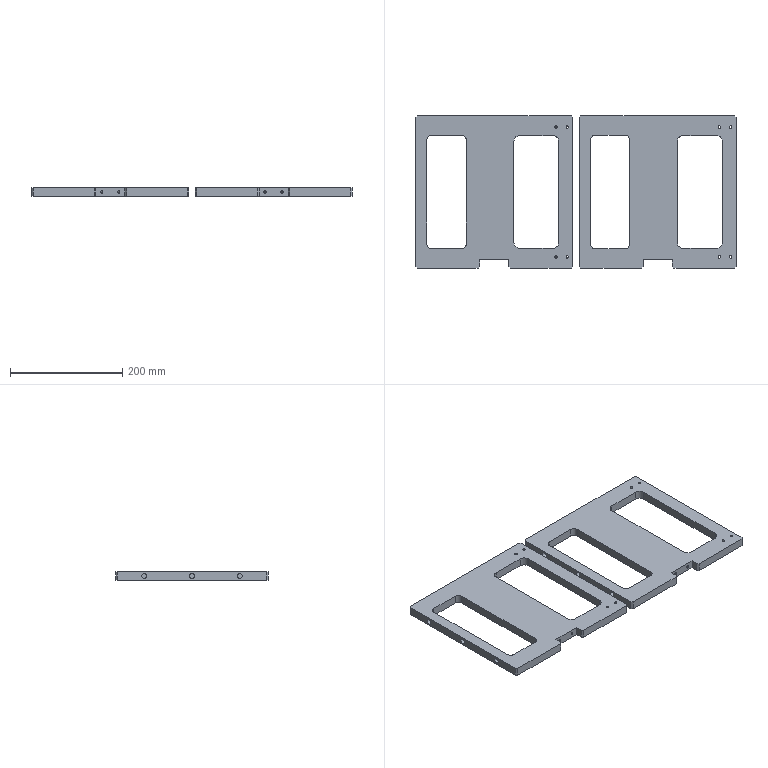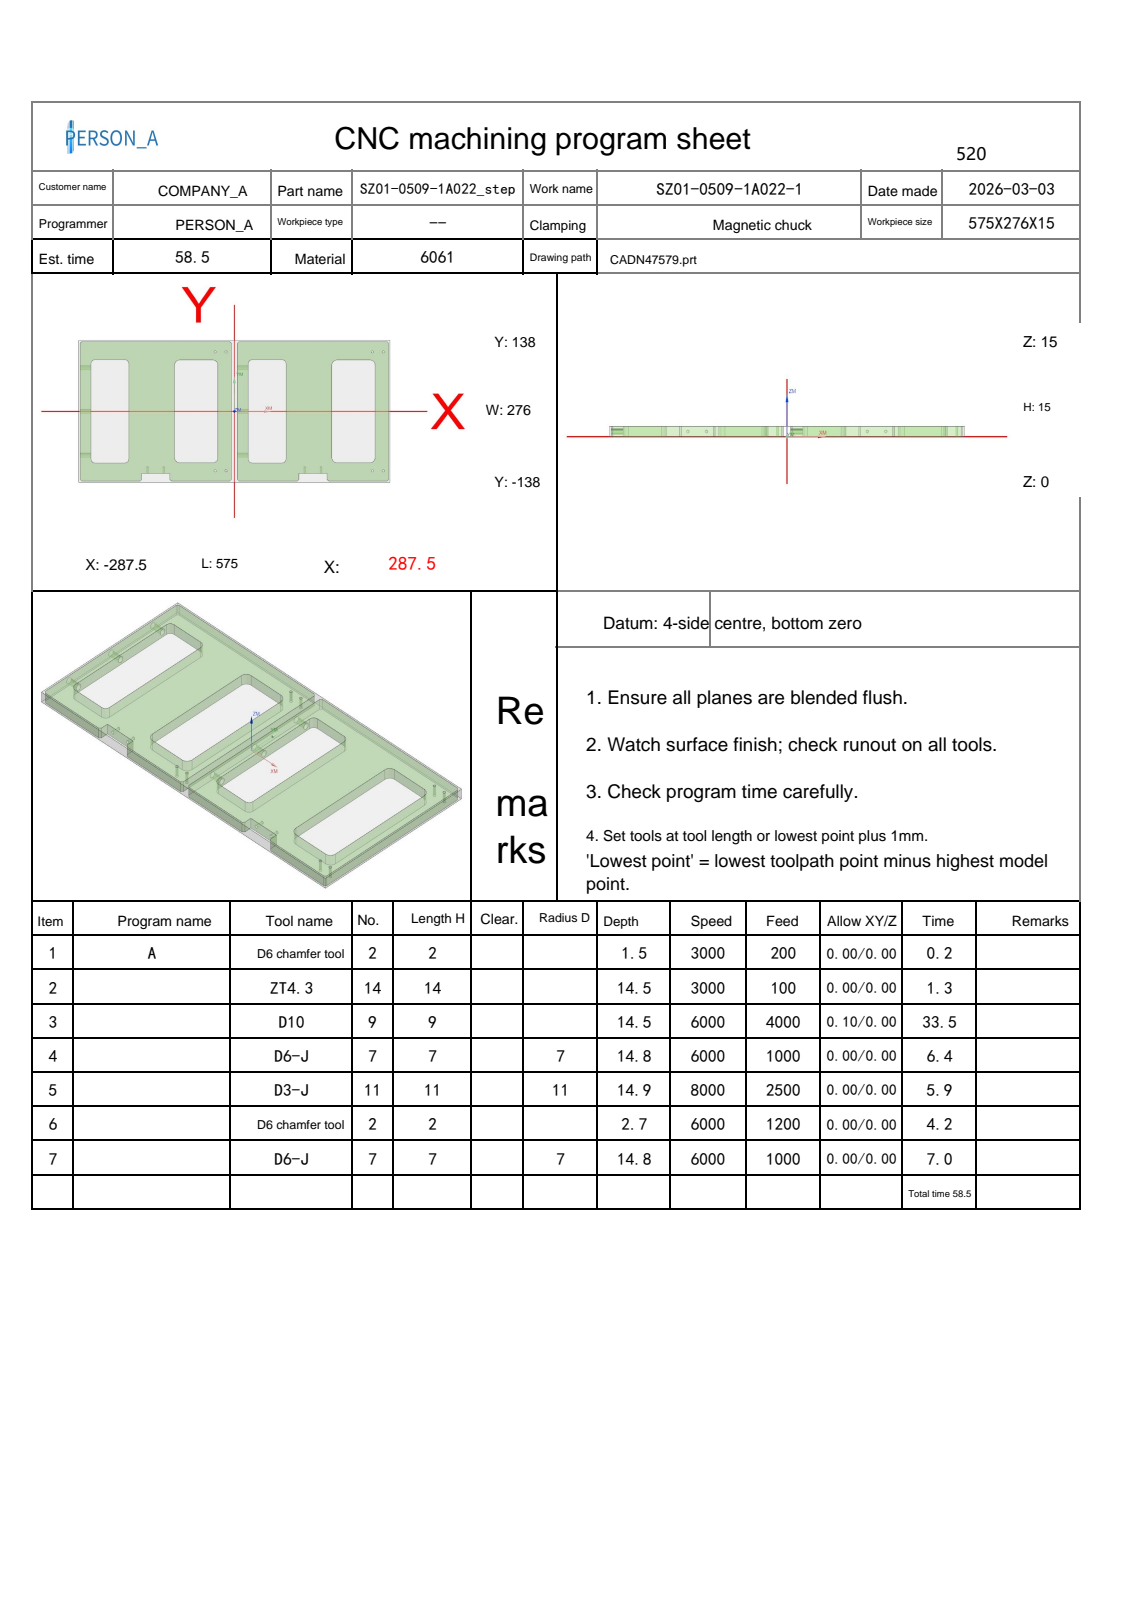NC program | NX | posted by the shop | part box 570 x 271 x 15 mm
Lines 2982 to 3815 of 10286:
N5 T11 M06
(D3-J  D=3. R=0. H=11 ce=0.00 di=0.00)
(D.N=11 MAX_Z=45. MIN_Z=0.15 Time=5.87M)
G00 G90 G54 X-15.613 Y114.911 M03 S8000
G43 H11 Z45.
M08
Z15.5
G01 X-15.578 Y114.9 Z15.498 F300.
X-15.422 Z15.49
X-15.233 Y114.957 Z15.48
X-15.072 Y115.072 Z15.469
X-14.957 Y115.233 Z15.459
X-14.9 Y115.422 Z15.448
Y115.578 Z15.44
X-14.953 Y115.758 Z15.43
X-15.059 Y115.914 Z15.421
X-15.208 Y116.03 Z15.411
X-15.385 Y116.094 Z15.401
X-15.578 Y116.1 Z15.391
X-15.767 Y116.043 Z15.38
X-15.928 Y115.928 Z15.37
X-16.043 Y115.767 Z15.36
X-16.1 Y115.578 Z15.349
Y115.422 Z15.341
X-16.043 Y115.233 Z15.331
X-15.928 Y115.072 Z15.32
X-15.767 Y114.957 Z15.31
X-15.578 Y114.9 Z15.3
X-15.422 Z15.292
X-15.233 Y114.957 Z15.281
X-15.072 Y115.072 Z15.271
X-14.957 Y115.233 Z15.26
X-14.9 Y115.422 Z15.25
Y115.578 Z15.242
X-14.953 Y115.758 Z15.232
X-15.059 Y115.914 Z15.222
X-15.208 Y116.03 Z15.212
X-15.385 Y116.094 Z15.202
X-15.578 Y116.1 Z15.192
X-15.767 Y116.043 Z15.182
X-15.928 Y115.928 Z15.172
X-16.043 Y115.767 Z15.161
X-16.1 Y115.578 Z15.151
Y115.422 Z15.143
X-16.043 Y115.233 Z15.132
X-15.928 Y115.072 Z15.122
X-15.767 Y114.957 Z15.112
X-15.578 Y114.9 Z15.101
X-15.422 Z15.093
X-15.233 Y114.957 Z15.083
X-15.072 Y115.072 Z15.072
X-14.957 Y115.233 Z15.062
X-14.9 Y115.422 Z15.052
Y115.578 Z15.044
X-14.953 Y115.758 Z15.034
X-15.059 Y115.914 Z15.024
X-15.208 Y116.03 Z15.014
X-15.385 Y116.094 Z15.004
X-15.463 Y116.099 Z15.
X-15.465 Y116.065
G41 D11
X-15.5 Y116.1
G03 X-16.1 Y115.5 Z14.914 I0.0 J-.6
X-15.5 Y114.9 Z14.827 I.6 J0.0
X-14.9 Y115.5 Z14.741 I0.0 J.6
X-15.5 Y116.1 Z14.655 I-.6 J0.0
X-16.1 Y115.5 Z14.568 I0.0 J-.6
X-15.5 Y114.9 Z14.482 I.6 J0.0
X-14.9 Y115.5 Z14.396 I0.0 J.6
X-15.5 Y116.1 Z14.309 I-.6 J0.0
X-16.1 Y115.5 Z14.223 I0.0 J-.6
X-15.5 Y114.9 Z14.137 I.6 J0.0
X-14.9 Y115.5 Z14.05 I0.0 J.6
X-15.5 Y116.1 Z13.964 I-.6 J0.0
X-16.1 Y115.5 Z13.878 I0.0 J-.6
X-15.5 Y114.9 Z13.791 I.6 J0.0
X-14.9 Y115.5 Z13.705 I0.0 J.6
X-15.5 Y116.1 Z13.619 I-.6 J0.0
X-16.1 Y115.5 Z13.532 I0.0 J-.6
X-15.5 Y114.9 Z13.446 I.6 J0.0
X-14.9 Y115.5 Z13.36 I0.0 J.6
X-15.5 Y116.1 Z13.273 I-.6 J0.0
X-16.1 Y115.5 Z13.187 I0.0 J-.6
X-15.5 Y114.9 Z13.101 I.6 J0.0
X-14.9 Y115.5 Z13.014 I0.0 J.6
X-15.5 Y116.1 Z12.928 I-.6 J0.0
X-16.1 Y115.5 Z12.842 I0.0 J-.6
X-15.5 Y114.9 Z12.755 I.6 J0.0
X-14.9 Y115.5 Z12.669 I0.0 J.6
X-15.5 Y116.1 Z12.583 I-.6 J0.0
X-16.1 Y115.5 Z12.496 I0.0 J-.6
X-15.5 Y114.9 Z12.41 I.6 J0.0
X-14.9 Y115.5 Z12.324 I0.0 J.6
X-15.5 Y116.1 Z12.237 I-.6 J0.0
X-16.1 Y115.5 Z12.151 I0.0 J-.6
X-15.5 Y114.9 Z12.065 I.6 J0.0
X-14.9 Y115.5 Z11.978 I0.0 J.6
X-15.5 Y116.1 Z11.892 I-.6 J0.0
X-16.1 Y115.5 Z11.806 I0.0 J-.6
X-15.5 Y114.9 Z11.719 I.6 J0.0
X-14.9 Y115.5 Z11.633 I0.0 J.6
X-15.5 Y116.1 Z11.547 I-.6 J0.0
X-16.1 Y115.5 Z11.46 I0.0 J-.6
X-15.5 Y114.9 Z11.374 I.6 J0.0
X-14.9 Y115.5 Z11.288 I0.0 J.6
X-15.5 Y116.1 Z11.201 I-.6 J0.0
X-16.1 Y115.5 Z11.115 I0.0 J-.6
X-15.5 Y114.9 Z11.028 I.6 J0.0
X-14.9 Y115.5 Z10.942 I0.0 J.6
X-15.5 Y116.1 Z10.856 I-.6 J0.0
X-16.1 Y115.5 Z10.769 I0.0 J-.6
X-15.5 Y114.9 Z10.683 I.6 J0.0
X-14.9 Y115.5 Z10.597 I0.0 J.6
X-15.5 Y116.1 Z10.51 I-.6 J0.0
X-16.1 Y115.5 Z10.424 I0.0 J-.6
X-15.5 Y114.9 Z10.338 I.6 J0.0
X-14.9 Y115.5 Z10.251 I0.0 J.6
X-15.5 Y116.1 Z10.165 I-.6 J0.0
X-16.1 Y115.5 Z10.079 I0.0 J-.6
X-15.5 Y114.9 Z9.992 I.6 J0.0
X-14.9 Y115.5 Z9.906 I0.0 J.6
X-15.5 Y116.1 Z9.82 I-.6 J0.0
X-16.1 Y115.5 Z9.733 I0.0 J-.6
X-15.5 Y114.9 Z9.647 I.6 J0.0
X-14.9 Y115.5 Z9.561 I0.0 J.6
X-15.5 Y116.1 Z9.474 I-.6 J0.0
X-16.1 Y115.5 Z9.388 I0.0 J-.6
X-15.5 Y114.9 Z9.302 I.6 J0.0
X-14.9 Y115.5 Z9.215 I0.0 J.6
X-15.5 Y116.1 Z9.129 I-.6 J0.0
X-16.1 Y115.5 Z9.043 I0.0 J-.6
X-15.5 Y114.9 Z8.956 I.6 J0.0
X-14.9 Y115.5 Z8.87 I0.0 J.6
X-15.5 Y116.1 Z8.784 I-.6 J0.0
X-16.1 Y115.5 Z8.697 I0.0 J-.6
X-15.5 Y114.9 Z8.611 I.6 J0.0
X-14.9 Y115.5 Z8.525 I0.0 J.6
X-15.5 Y116.1 Z8.438 I-.6 J0.0
X-16.1 Y115.5 Z8.352 I0.0 J-.6
X-15.5 Y114.9 Z8.266 I.6 J0.0
X-14.9 Y115.5 Z8.179 I0.0 J.6
X-15.5 Y116.1 Z8.093 I-.6 J0.0
X-16.1 Y115.5 Z8.007 I0.0 J-.6
X-15.5 Y114.9 Z7.92 I.6 J0.0
X-14.9 Y115.5 Z7.834 I0.0 J.6
X-15.5 Y116.1 Z7.748 I-.6 J0.0
X-16.1 Y115.5 Z7.661 I0.0 J-.6
X-15.5 Y114.9 Z7.575 I.6 J0.0
X-14.9 Y115.5 Z7.489 I0.0 J.6
X-15.5 Y116.1 Z7.402 I-.6 J0.0
X-16.1 Y115.5 Z7.316 I0.0 J-.6
X-15.5 Y114.9 Z7.23 I.6 J0.0
X-14.9 Y115.5 Z7.143 I0.0 J.6
X-15.5 Y116.1 Z7.057 I-.6 J0.0
X-16.1 Y115.5 Z6.971 I0.0 J-.6
X-15.5 Y114.9 Z6.884 I.6 J0.0
X-14.9 Y115.5 Z6.798 I0.0 J.6
X-15.5 Y116.1 Z6.712 I-.6 J0.0
X-16.1 Y115.5 Z6.625 I0.0 J-.6
X-15.5 Y114.9 Z6.539 I.6 J0.0
X-14.9 Y115.5 Z6.453 I0.0 J.6
X-15.5 Y116.1 Z6.366 I-.6 J0.0
X-16.1 Y115.5 Z6.28 I0.0 J-.6
X-15.5 Y114.9 Z6.194 I.6 J0.0
X-14.9 Y115.5 Z6.107 I0.0 J.6
X-15.5 Y116.1 Z6.021 I-.6 J0.0
X-16.1 Y115.5 Z5.935 I0.0 J-.6
X-15.5 Y114.9 Z5.848 I.6 J0.0
X-14.9 Y115.5 Z5.762 I0.0 J.6
X-15.5 Y116.1 Z5.676 I-.6 J0.0
X-16.1 Y115.5 Z5.589 I0.0 J-.6
X-15.5 Y114.9 Z5.503 I.6 J0.0
X-14.9 Y115.5 Z5.417 I0.0 J.6
X-15.5 Y116.1 Z5.33 I-.6 J0.0
X-16.1 Y115.5 Z5.244 I0.0 J-.6
X-15.5 Y114.9 Z5.158 I.6 J0.0
X-14.9 Y115.5 Z5.071 I0.0 J.6
X-15.5 Y116.1 Z4.985 I-.6 J0.0
X-16.1 Y115.5 Z4.899 I0.0 J-.6
X-15.5 Y114.9 Z4.812 I.6 J0.0
X-14.9 Y115.5 Z4.726 I0.0 J.6
X-15.5 Y116.1 Z4.64 I-.6 J0.0
X-16.1 Y115.5 Z4.553 I0.0 J-.6
X-15.5 Y114.9 Z4.467 I.6 J0.0
X-14.9 Y115.5 Z4.381 I0.0 J.6
X-15.5 Y116.1 Z4.294 I-.6 J0.0
X-16.1 Y115.5 Z4.208 I0.0 J-.6
X-15.5 Y114.9 Z4.122 I.6 J0.0
X-14.9 Y115.5 Z4.035 I0.0 J.6
X-15.5 Y116.1 Z3.949 I-.6 J0.0
X-16.1 Y115.5 Z3.863 I0.0 J-.6
X-15.5 Y114.9 Z3.776 I.6 J0.0
X-14.9 Y115.5 Z3.69 I0.0 J.6
X-15.5 Y116.1 Z3.603 I-.6 J0.0
X-16.1 Y115.5 Z3.517 I0.0 J-.6
X-15.5 Y114.9 Z3.431 I.6 J0.0
X-14.9 Y115.5 Z3.344 I0.0 J.6
X-15.5 Y116.1 Z3.258 I-.6 J0.0
X-16.1 Y115.5 Z3.172 I0.0 J-.6
X-15.5 Y114.9 Z3.085 I.6 J0.0
X-14.9 Y115.5 Z2.999 I0.0 J.6
X-15.5 Y116.1 Z2.913 I-.6 J0.0
X-16.1 Y115.5 Z2.826 I0.0 J-.6
X-15.5 Y114.9 Z2.74 I.6 J0.0
X-14.9 Y115.5 Z2.654 I0.0 J.6
X-15.5 Y116.1 Z2.567 I-.6 J0.0
X-16.1 Y115.5 Z2.481 I0.0 J-.6
X-15.5 Y114.9 Z2.395 I.6 J0.0
X-14.9 Y115.5 Z2.308 I0.0 J.6
X-15.5 Y116.1 Z2.222 I-.6 J0.0
X-16.1 Y115.5 Z2.136 I0.0 J-.6
X-15.5 Y114.9 Z2.049 I.6 J0.0
X-14.9 Y115.5 Z1.963 I0.0 J.6
X-15.5 Y116.1 Z1.877 I-.6 J0.0
X-16.1 Y115.5 Z1.79 I0.0 J-.6
X-15.5 Y114.9 Z1.704 I.6 J0.0
X-14.9 Y115.5 Z1.618 I0.0 J.6
X-15.5 Y116.1 Z1.531 I-.6 J0.0
X-16.1 Y115.5 Z1.445 I0.0 J-.6
X-15.5 Y114.9 Z1.359 I.6 J0.0
X-14.9 Y115.5 Z1.272 I0.0 J.6
X-15.5 Y116.1 Z1.186 I-.6 J0.0
X-16.1 Y115.5 Z1.1 I0.0 J-.6
X-15.5 Y114.9 Z1.013 I.6 J0.0
X-14.9 Y115.5 Z.927 I0.0 J.6
X-15.5 Y116.1 Z.841 I-.6 J0.0
X-16.1 Y115.5 Z.754 I0.0 J-.6
X-15.5 Y114.9 Z.668 I.6 J0.0
X-14.9 Y115.5 Z.582 I0.0 J.6
X-15.5 Y116.1 Z.495 I-.6 J0.0
X-16.1 Y115.5 Z.409 I0.0 J-.6
X-15.5 Y114.9 Z.323 I.6 J0.0
X-14.9 Y115.5 Z.236 I0.0 J.6
X-15.5 Y116.1 Z.15 I-.6 J0.0
X-16.1 Y115.5 I0.0 J-.6
X-15.5 Y114.9 I.6 J0.0
X-14.9 Y115.5 I0.0 J.6
X-15.5 Y116.1 I-.6 J0.0
X-15.871 Y115.972 I0.0 J-.6
G01 X-15.891 Y115.953
X-15.895 Y115.924
X-15.879 Y115.901
G40 X-15.848 Y115.862
Z1.15
G00 Z45.
X-35.613 Y114.911
Z15.5
G01 X-35.578 Y114.9 Z15.498
X-35.422 Z15.49
X-35.233 Y114.957 Z15.48
X-35.072 Y115.072 Z15.469
X-34.957 Y115.233 Z15.459
X-34.9 Y115.422 Z15.448
Y115.578 Z15.44
X-34.953 Y115.758 Z15.43
X-35.059 Y115.914 Z15.421
X-35.208 Y116.03 Z15.411
X-35.385 Y116.094 Z15.401
X-35.578 Y116.1 Z15.391
X-35.767 Y116.043 Z15.38
X-35.928 Y115.928 Z15.37
X-36.043 Y115.767 Z15.36
X-36.1 Y115.578 Z15.349
Y115.422 Z15.341
X-36.043 Y115.233 Z15.331
X-35.928 Y115.072 Z15.32
X-35.767 Y114.957 Z15.31
X-35.578 Y114.9 Z15.3
X-35.422 Z15.292
X-35.233 Y114.957 Z15.281
X-35.072 Y115.072 Z15.271
X-34.957 Y115.233 Z15.26
X-34.9 Y115.422 Z15.25
Y115.578 Z15.242
X-34.953 Y115.758 Z15.232
X-35.059 Y115.914 Z15.222
X-35.208 Y116.03 Z15.212
X-35.385 Y116.094 Z15.202
X-35.578 Y116.1 Z15.192
X-35.767 Y116.043 Z15.182
X-35.928 Y115.928 Z15.172
X-36.043 Y115.767 Z15.161
X-36.1 Y115.578 Z15.151
Y115.422 Z15.143
X-36.043 Y115.233 Z15.132
X-35.928 Y115.072 Z15.122
X-35.767 Y114.957 Z15.112
X-35.578 Y114.9 Z15.101
X-35.422 Z15.093
X-35.233 Y114.957 Z15.083
X-35.072 Y115.072 Z15.072
X-34.957 Y115.233 Z15.062
X-34.9 Y115.422 Z15.052
Y115.578 Z15.044
X-34.953 Y115.758 Z15.034
X-35.059 Y115.914 Z15.024
X-35.208 Y116.03 Z15.014
X-35.385 Y116.094 Z15.004
X-35.463 Y116.099 Z15.
X-35.465 Y116.065
G41 D11
X-35.5 Y116.1
G03 X-36.1 Y115.5 Z14.914 I0.0 J-.6
X-35.5 Y114.9 Z14.827 I.6 J0.0
X-34.9 Y115.5 Z14.741 I0.0 J.6
X-35.5 Y116.1 Z14.655 I-.6 J0.0
X-36.1 Y115.5 Z14.568 I0.0 J-.6
X-35.5 Y114.9 Z14.482 I.6 J0.0
X-34.9 Y115.5 Z14.396 I0.0 J.6
X-35.5 Y116.1 Z14.309 I-.6 J0.0
X-36.1 Y115.5 Z14.223 I0.0 J-.6
X-35.5 Y114.9 Z14.137 I.6 J0.0
X-34.9 Y115.5 Z14.05 I0.0 J.6
X-35.5 Y116.1 Z13.964 I-.6 J0.0
X-36.1 Y115.5 Z13.878 I0.0 J-.6
X-35.5 Y114.9 Z13.791 I.6 J0.0
X-34.9 Y115.5 Z13.705 I0.0 J.6
X-35.5 Y116.1 Z13.619 I-.6 J0.0
X-36.1 Y115.5 Z13.532 I0.0 J-.6
X-35.5 Y114.9 Z13.446 I.6 J0.0
X-34.9 Y115.5 Z13.36 I0.0 J.6
X-35.5 Y116.1 Z13.273 I-.6 J0.0
X-36.1 Y115.5 Z13.187 I0.0 J-.6
X-35.5 Y114.9 Z13.101 I.6 J0.0
X-34.9 Y115.5 Z13.014 I0.0 J.6
X-35.5 Y116.1 Z12.928 I-.6 J0.0
X-36.1 Y115.5 Z12.842 I0.0 J-.6
X-35.5 Y114.9 Z12.755 I.6 J0.0
X-34.9 Y115.5 Z12.669 I0.0 J.6
X-35.5 Y116.1 Z12.583 I-.6 J0.0
X-36.1 Y115.5 Z12.496 I0.0 J-.6
X-35.5 Y114.9 Z12.41 I.6 J0.0
X-34.9 Y115.5 Z12.324 I0.0 J.6
X-35.5 Y116.1 Z12.237 I-.6 J0.0
X-36.1 Y115.5 Z12.151 I0.0 J-.6
X-35.5 Y114.9 Z12.065 I.6 J0.0
X-34.9 Y115.5 Z11.978 I0.0 J.6
X-35.5 Y116.1 Z11.892 I-.6 J0.0
X-36.1 Y115.5 Z11.806 I0.0 J-.6
X-35.5 Y114.9 Z11.719 I.6 J0.0
X-34.9 Y115.5 Z11.633 I0.0 J.6
X-35.5 Y116.1 Z11.547 I-.6 J0.0
X-36.1 Y115.5 Z11.46 I0.0 J-.6
X-35.5 Y114.9 Z11.374 I.6 J0.0
X-34.9 Y115.5 Z11.288 I0.0 J.6
X-35.5 Y116.1 Z11.201 I-.6 J0.0
X-36.1 Y115.5 Z11.115 I0.0 J-.6
X-35.5 Y114.9 Z11.028 I.6 J0.0
X-34.9 Y115.5 Z10.942 I0.0 J.6
X-35.5 Y116.1 Z10.856 I-.6 J0.0
X-36.1 Y115.5 Z10.769 I0.0 J-.6
X-35.5 Y114.9 Z10.683 I.6 J0.0
X-34.9 Y115.5 Z10.597 I0.0 J.6
X-35.5 Y116.1 Z10.51 I-.6 J0.0
X-36.1 Y115.5 Z10.424 I0.0 J-.6
X-35.5 Y114.9 Z10.338 I.6 J0.0
X-34.9 Y115.5 Z10.251 I0.0 J.6
X-35.5 Y116.1 Z10.165 I-.6 J0.0
X-36.1 Y115.5 Z10.079 I0.0 J-.6
X-35.5 Y114.9 Z9.992 I.6 J0.0
X-34.9 Y115.5 Z9.906 I0.0 J.6
X-35.5 Y116.1 Z9.82 I-.6 J0.0
X-36.1 Y115.5 Z9.733 I0.0 J-.6
X-35.5 Y114.9 Z9.647 I.6 J0.0
X-34.9 Y115.5 Z9.561 I0.0 J.6
X-35.5 Y116.1 Z9.474 I-.6 J0.0
X-36.1 Y115.5 Z9.388 I0.0 J-.6
X-35.5 Y114.9 Z9.302 I.6 J0.0
X-34.9 Y115.5 Z9.215 I0.0 J.6
X-35.5 Y116.1 Z9.129 I-.6 J0.0
X-36.1 Y115.5 Z9.043 I0.0 J-.6
X-35.5 Y114.9 Z8.956 I.6 J0.0
X-34.9 Y115.5 Z8.87 I0.0 J.6
X-35.5 Y116.1 Z8.784 I-.6 J0.0
X-36.1 Y115.5 Z8.697 I0.0 J-.6
X-35.5 Y114.9 Z8.611 I.6 J0.0
X-34.9 Y115.5 Z8.525 I0.0 J.6
X-35.5 Y116.1 Z8.438 I-.6 J0.0
X-36.1 Y115.5 Z8.352 I0.0 J-.6
X-35.5 Y114.9 Z8.266 I.6 J0.0
X-34.9 Y115.5 Z8.179 I0.0 J.6
X-35.5 Y116.1 Z8.093 I-.6 J0.0
X-36.1 Y115.5 Z8.007 I0.0 J-.6
X-35.5 Y114.9 Z7.92 I.6 J0.0
X-34.9 Y115.5 Z7.834 I0.0 J.6
X-35.5 Y116.1 Z7.748 I-.6 J0.0
X-36.1 Y115.5 Z7.661 I0.0 J-.6
X-35.5 Y114.9 Z7.575 I.6 J0.0
X-34.9 Y115.5 Z7.489 I0.0 J.6
X-35.5 Y116.1 Z7.402 I-.6 J0.0
X-36.1 Y115.5 Z7.316 I0.0 J-.6
X-35.5 Y114.9 Z7.23 I.6 J0.0
X-34.9 Y115.5 Z7.143 I0.0 J.6
X-35.5 Y116.1 Z7.057 I-.6 J0.0
X-36.1 Y115.5 Z6.971 I0.0 J-.6
X-35.5 Y114.9 Z6.884 I.6 J0.0
X-34.9 Y115.5 Z6.798 I0.0 J.6
X-35.5 Y116.1 Z6.712 I-.6 J0.0
X-36.1 Y115.5 Z6.625 I0.0 J-.6
X-35.5 Y114.9 Z6.539 I.6 J0.0
X-34.9 Y115.5 Z6.453 I0.0 J.6
X-35.5 Y116.1 Z6.366 I-.6 J0.0
X-36.1 Y115.5 Z6.28 I0.0 J-.6
X-35.5 Y114.9 Z6.194 I.6 J0.0
X-34.9 Y115.5 Z6.107 I0.0 J.6
X-35.5 Y116.1 Z6.021 I-.6 J0.0
X-36.1 Y115.5 Z5.935 I0.0 J-.6
X-35.5 Y114.9 Z5.848 I.6 J0.0
X-34.9 Y115.5 Z5.762 I0.0 J.6
X-35.5 Y116.1 Z5.676 I-.6 J0.0
X-36.1 Y115.5 Z5.589 I0.0 J-.6
X-35.5 Y114.9 Z5.503 I.6 J0.0
X-34.9 Y115.5 Z5.417 I0.0 J.6
X-35.5 Y116.1 Z5.33 I-.6 J0.0
X-36.1 Y115.5 Z5.244 I0.0 J-.6
X-35.5 Y114.9 Z5.158 I.6 J0.0
X-34.9 Y115.5 Z5.071 I0.0 J.6
X-35.5 Y116.1 Z4.985 I-.6 J0.0
X-36.1 Y115.5 Z4.899 I0.0 J-.6
X-35.5 Y114.9 Z4.812 I.6 J0.0
X-34.9 Y115.5 Z4.726 I0.0 J.6
X-35.5 Y116.1 Z4.64 I-.6 J0.0
X-36.1 Y115.5 Z4.553 I0.0 J-.6
X-35.5 Y114.9 Z4.467 I.6 J0.0
X-34.9 Y115.5 Z4.381 I0.0 J.6
X-35.5 Y116.1 Z4.294 I-.6 J0.0
X-36.1 Y115.5 Z4.208 I0.0 J-.6
X-35.5 Y114.9 Z4.122 I.6 J0.0
X-34.9 Y115.5 Z4.035 I0.0 J.6
X-35.5 Y116.1 Z3.949 I-.6 J0.0
X-36.1 Y115.5 Z3.863 I0.0 J-.6
X-35.5 Y114.9 Z3.776 I.6 J0.0
X-34.9 Y115.5 Z3.69 I0.0 J.6
X-35.5 Y116.1 Z3.603 I-.6 J0.0
X-36.1 Y115.5 Z3.517 I0.0 J-.6
X-35.5 Y114.9 Z3.431 I.6 J0.0
X-34.9 Y115.5 Z3.344 I0.0 J.6
X-35.5 Y116.1 Z3.258 I-.6 J0.0
X-36.1 Y115.5 Z3.172 I0.0 J-.6
X-35.5 Y114.9 Z3.085 I.6 J0.0
X-34.9 Y115.5 Z2.999 I0.0 J.6
X-35.5 Y116.1 Z2.913 I-.6 J0.0
X-36.1 Y115.5 Z2.826 I0.0 J-.6
X-35.5 Y114.9 Z2.74 I.6 J0.0
X-34.9 Y115.5 Z2.654 I0.0 J.6
X-35.5 Y116.1 Z2.567 I-.6 J0.0
X-36.1 Y115.5 Z2.481 I0.0 J-.6
X-35.5 Y114.9 Z2.395 I.6 J0.0
X-34.9 Y115.5 Z2.308 I0.0 J.6
X-35.5 Y116.1 Z2.222 I-.6 J0.0
X-36.1 Y115.5 Z2.136 I0.0 J-.6
X-35.5 Y114.9 Z2.049 I.6 J0.0
X-34.9 Y115.5 Z1.963 I0.0 J.6
X-35.5 Y116.1 Z1.877 I-.6 J0.0
X-36.1 Y115.5 Z1.79 I0.0 J-.6
X-35.5 Y114.9 Z1.704 I.6 J0.0
X-34.9 Y115.5 Z1.618 I0.0 J.6
X-35.5 Y116.1 Z1.531 I-.6 J0.0
X-36.1 Y115.5 Z1.445 I0.0 J-.6
X-35.5 Y114.9 Z1.359 I.6 J0.0
X-34.9 Y115.5 Z1.272 I0.0 J.6
X-35.5 Y116.1 Z1.186 I-.6 J0.0
X-36.1 Y115.5 Z1.1 I0.0 J-.6
X-35.5 Y114.9 Z1.013 I.6 J0.0
X-34.9 Y115.5 Z.927 I0.0 J.6
X-35.5 Y116.1 Z.841 I-.6 J0.0
X-36.1 Y115.5 Z.754 I0.0 J-.6
X-35.5 Y114.9 Z.668 I.6 J0.0
X-34.9 Y115.5 Z.582 I0.0 J.6
X-35.5 Y116.1 Z.495 I-.6 J0.0
X-36.1 Y115.5 Z.409 I0.0 J-.6
X-35.5 Y114.9 Z.323 I.6 J0.0
X-34.9 Y115.5 Z.236 I0.0 J.6
X-35.5 Y116.1 Z.15 I-.6 J0.0
X-36.1 Y115.5 I0.0 J-.6
X-35.5 Y114.9 I.6 J0.0
X-34.9 Y115.5 I0.0 J.6
X-35.5 Y116.1 I-.6 J0.0
X-35.871 Y115.972 I0.0 J-.6
G01 X-35.891 Y115.953
X-35.895 Y115.924
X-35.879 Y115.901
G40 X-35.848 Y115.862
Z1.15
G00 Z45.
X-35.39 Y-114.91
Z15.5
G01 X-35.422 Y-114.9 Z15.498
X-35.578 Z15.49
X-35.767 Y-114.957 Z15.48
X-35.928 Y-115.072 Z15.469
X-36.043 Y-115.233 Z15.459
X-36.1 Y-115.422 Z15.449
Y-115.578 Z15.441
X-36.069 Y-115.707 Z15.434
X-36.01 Y-115.826 Z15.427
X-35.91 Y-115.945 Z15.418
X-35.773 Y-116.04 Z15.41
X-35.615 Y-116.094 Z15.401
X-35.422 Y-116.1 Z15.391
X-35.233 Y-116.043 Z15.38
X-35.072 Y-115.928 Z15.37
X-34.957 Y-115.767 Z15.36
X-34.9 Y-115.578 Z15.349
Y-115.422 Z15.341
X-34.957 Y-115.233 Z15.331
X-35.072 Y-115.072 Z15.321
X-35.233 Y-114.957 Z15.31
X-35.422 Y-114.9 Z15.3
X-35.578 Z15.292
X-35.767 Y-114.957 Z15.281
X-35.928 Y-115.072 Z15.271
X-36.043 Y-115.233 Z15.261
X-36.1 Y-115.422 Z15.25
Y-115.578 Z15.242
X-36.069 Y-115.707 Z15.235
X-36.01 Y-115.826 Z15.228
X-35.91 Y-115.945 Z15.22
X-35.773 Y-116.04 Z15.211
X-35.615 Y-116.094 Z15.203
X-35.422 Y-116.1 Z15.192
X-35.233 Y-116.043 Z15.182
X-35.072 Y-115.928 Z15.172
X-34.957 Y-115.767 Z15.161
X-34.9 Y-115.578 Z15.151
Y-115.422 Z15.143
X-34.957 Y-115.233 Z15.132
X-35.072 Y-115.072 Z15.122
X-35.233 Y-114.957 Z15.112
X-35.422 Y-114.9 Z15.101
X-35.578 Z15.093
X-35.767 Y-114.957 Z15.083
X-35.928 Y-115.072 Z15.072
X-36.043 Y-115.233 Z15.062
X-36.1 Y-115.422 Z15.052
Y-115.578 Z15.044
X-36.069 Y-115.707 Z15.037
X-36.01 Y-115.826 Z15.03
X-35.91 Y-115.945 Z15.022
X-35.773 Y-116.04 Z15.013
X-35.615 Y-116.094 Z15.004
X-35.537 Y-116.099 Z15.
X-35.535 Y-116.065
G41 D11
X-35.5 Y-116.1
G03 X-34.9 Y-115.5 Z14.914 I0.0 J.6
X-35.5 Y-114.9 Z14.827 I-.6 J0.0
X-36.1 Y-115.5 Z14.741 I0.0 J-.6
X-35.96 Y-115.885 Z14.703 I.6 J0.0
X-35.5 Y-116.1 Z14.655 I.46 J.385
X-34.9 Y-115.5 Z14.568 I0.0 J.6
X-35.5 Y-114.9 Z14.482 I-.6 J0.0
X-36.1 Y-115.5 Z14.396 I0.0 J-.6
X-35.96 Y-115.885 Z14.357 I.6 J0.0
X-35.5 Y-116.1 Z14.309 I.46 J.385
X-34.9 Y-115.5 Z14.223 I0.0 J.6
X-35.5 Y-114.9 Z14.137 I-.6 J0.0
X-36.1 Y-115.5 Z14.05 I0.0 J-.6
X-35.96 Y-115.885 Z14.012 I.6 J0.0
X-35.5 Y-116.1 Z13.964 I.46 J.385
X-34.9 Y-115.5 Z13.878 I0.0 J.6
X-35.5 Y-114.9 Z13.791 I-.6 J0.0
X-36.1 Y-115.5 Z13.705 I0.0 J-.6
X-35.96 Y-115.885 Z13.667 I.6 J0.0
X-35.5 Y-116.1 Z13.619 I.46 J.385
X-34.9 Y-115.5 Z13.532 I0.0 J.6
X-35.5 Y-114.9 Z13.446 I-.6 J0.0
X-36.1 Y-115.5 Z13.36 I0.0 J-.6
X-35.96 Y-115.885 Z13.321 I.6 J0.0
X-35.5 Y-116.1 Z13.273 I.46 J.385
X-34.9 Y-115.5 Z13.187 I0.0 J.6
X-35.5 Y-114.9 Z13.101 I-.6 J0.0
X-36.1 Y-115.5 Z13.014 I0.0 J-.6
X-35.96 Y-115.885 Z12.976 I.6 J0.0
X-35.5 Y-116.1 Z12.928 I.46 J.385
X-34.9 Y-115.5 Z12.842 I0.0 J.6
X-35.5 Y-114.9 Z12.755 I-.6 J0.0
X-36.1 Y-115.5 Z12.669 I0.0 J-.6
X-35.96 Y-115.885 Z12.631 I.6 J0.0
X-35.5 Y-116.1 Z12.583 I.46 J.385
X-34.9 Y-115.5 Z12.496 I0.0 J.6
X-35.5 Y-114.9 Z12.41 I-.6 J0.0
X-36.1 Y-115.5 Z12.324 I0.0 J-.6
X-35.96 Y-115.885 Z12.285 I.6 J0.0
X-35.5 Y-116.1 Z12.237 I.46 J.385
X-34.9 Y-115.5 Z12.151 I0.0 J.6
X-35.5 Y-114.9 Z12.065 I-.6 J0.0
X-36.1 Y-115.5 Z11.978 I0.0 J-.6
X-35.96 Y-115.885 Z11.94 I.6 J0.0
X-35.5 Y-116.1 Z11.892 I.46 J.385
X-34.9 Y-115.5 Z11.806 I0.0 J.6
X-35.5 Y-114.9 Z11.719 I-.6 J0.0
X-36.1 Y-115.5 Z11.633 I0.0 J-.6
X-35.96 Y-115.885 Z11.595 I.6 J0.0
X-35.5 Y-116.1 Z11.547 I.46 J.385
X-34.9 Y-115.5 Z11.46 I0.0 J.6
X-35.5 Y-114.9 Z11.374 I-.6 J0.0
X-36.1 Y-115.5 Z11.288 I0.0 J-.6
X-35.96 Y-115.885 Z11.249 I.6 J0.0
X-35.5 Y-116.1 Z11.201 I.46 J.385
X-34.9 Y-115.5 Z11.115 I0.0 J.6
X-35.5 Y-114.9 Z11.028 I-.6 J0.0
X-36.1 Y-115.5 Z10.942 I0.0 J-.6
X-35.96 Y-115.885 Z10.904 I.6 J0.0
X-35.5 Y-116.1 Z10.856 I.46 J.385
X-34.9 Y-115.5 Z10.769 I0.0 J.6
X-35.5 Y-114.9 Z10.683 I-.6 J0.0
X-36.1 Y-115.5 Z10.597 I0.0 J-.6
X-35.96 Y-115.885 Z10.559 I.6 J0.0
X-35.5 Y-116.1 Z10.51 I.46 J.385
X-34.9 Y-115.5 Z10.424 I0.0 J.6
X-35.5 Y-114.9 Z10.338 I-.6 J0.0
X-36.1 Y-115.5 Z10.251 I0.0 J-.6
X-35.96 Y-115.885 Z10.213 I.6 J0.0
X-35.5 Y-116.1 Z10.165 I.46 J.385
X-34.9 Y-115.5 Z10.079 I0.0 J.6
X-35.5 Y-114.9 Z9.992 I-.6 J0.0
X-36.1 Y-115.5 Z9.906 I0.0 J-.6
X-35.96 Y-115.885 Z9.868 I.6 J0.0
X-35.5 Y-116.1 Z9.82 I.46 J.385
X-34.9 Y-115.5 Z9.733 I0.0 J.6
X-35.5 Y-114.9 Z9.647 I-.6 J0.0
X-36.1 Y-115.5 Z9.561 I0.0 J-.6
X-35.96 Y-115.885 Z9.522 I.6 J0.0
X-35.5 Y-116.1 Z9.474 I.46 J.385
X-34.9 Y-115.5 Z9.388 I0.0 J.6
X-35.5 Y-114.9 Z9.302 I-.6 J0.0
X-36.1 Y-115.5 Z9.215 I0.0 J-.6
X-35.96 Y-115.885 Z9.177 I.6 J0.0
X-35.5 Y-116.1 Z9.129 I.46 J.385
X-34.9 Y-115.5 Z9.043 I0.0 J.6
X-35.5 Y-114.9 Z8.956 I-.6 J0.0
X-36.1 Y-115.5 Z8.87 I0.0 J-.6
X-35.96 Y-115.885 Z8.832 I.6 J0.0
X-35.5 Y-116.1 Z8.784 I.46 J.385
X-34.9 Y-115.5 Z8.697 I0.0 J.6
X-35.5 Y-114.9 Z8.611 I-.6 J0.0
X-36.1 Y-115.5 Z8.525 I0.0 J-.6
X-35.96 Y-115.885 Z8.486 I.6 J0.0
X-35.5 Y-116.1 Z8.438 I.46 J.385
X-34.9 Y-115.5 Z8.352 I0.0 J.6
X-35.5 Y-114.9 Z8.266 I-.6 J0.0
X-36.1 Y-115.5 Z8.179 I0.0 J-.6
X-35.96 Y-115.885 Z8.141 I.6 J0.0
X-35.5 Y-116.1 Z8.093 I.46 J.385
X-34.9 Y-115.5 Z8.007 I0.0 J.6
X-35.5 Y-114.9 Z7.92 I-.6 J0.0
X-36.1 Y-115.5 Z7.834 I0.0 J-.6
X-35.96 Y-115.885 Z7.796 I.6 J0.0
X-35.5 Y-116.1 Z7.748 I.46 J.385
X-34.9 Y-115.5 Z7.661 I0.0 J.6
X-35.5 Y-114.9 Z7.575 I-.6 J0.0
X-36.1 Y-115.5 Z7.489 I0.0 J-.6
X-35.96 Y-115.885 Z7.45 I.6 J0.0
X-35.5 Y-116.1 Z7.402 I.46 J.385
X-34.9 Y-115.5 Z7.316 I0.0 J.6
X-35.5 Y-114.9 Z7.23 I-.6 J0.0
X-36.1 Y-115.5 Z7.143 I0.0 J-.6
X-35.96 Y-115.885 Z7.105 I.6 J0.0
X-35.5 Y-116.1 Z7.057 I.46 J.385
X-34.9 Y-115.5 Z6.971 I0.0 J.6
X-35.5 Y-114.9 Z6.884 I-.6 J0.0
X-36.1 Y-115.5 Z6.798 I0.0 J-.6
X-35.96 Y-115.885 Z6.76 I.6 J0.0
X-35.5 Y-116.1 Z6.712 I.46 J.385
X-34.9 Y-115.5 Z6.625 I0.0 J.6
X-35.5 Y-114.9 Z6.539 I-.6 J0.0
X-36.1 Y-115.5 Z6.453 I0.0 J-.6
X-35.96 Y-115.885 Z6.414 I.6 J0.0
X-35.5 Y-116.1 Z6.366 I.46 J.385
X-34.9 Y-115.5 Z6.28 I0.0 J.6
X-35.5 Y-114.9 Z6.194 I-.6 J0.0
X-36.1 Y-115.5 Z6.107 I0.0 J-.6
X-35.96 Y-115.885 Z6.069 I.6 J0.0
X-35.5 Y-116.1 Z6.021 I.46 J.385
X-34.9 Y-115.5 Z5.935 I0.0 J.6
X-35.5 Y-114.9 Z5.848 I-.6 J0.0
X-36.1 Y-115.5 Z5.762 I0.0 J-.6
X-35.96 Y-115.885 Z5.724 I.6 J0.0
X-35.5 Y-116.1 Z5.676 I.46 J.385
X-34.9 Y-115.5 Z5.589 I0.0 J.6
X-35.5 Y-114.9 Z5.503 I-.6 J0.0
X-36.1 Y-115.5 Z5.417 I0.0 J-.6
X-35.96 Y-115.885 Z5.378 I.6 J0.0
X-35.5 Y-116.1 Z5.33 I.46 J.385
X-34.9 Y-115.5 Z5.244 I0.0 J.6
X-35.5 Y-114.9 Z5.158 I-.6 J0.0
X-36.1 Y-115.5 Z5.071 I0.0 J-.6
X-35.96 Y-115.885 Z5.033 I.6 J0.0
X-35.5 Y-116.1 Z4.985 I.46 J.385
X-34.9 Y-115.5 Z4.899 I0.0 J.6
X-35.5 Y-114.9 Z4.812 I-.6 J0.0
X-36.1 Y-115.5 Z4.726 I0.0 J-.6
X-35.96 Y-115.885 Z4.688 I.6 J0.0
X-35.5 Y-116.1 Z4.64 I.46 J.385
X-34.9 Y-115.5 Z4.553 I0.0 J.6
X-35.5 Y-114.9 Z4.467 I-.6 J0.0
X-36.1 Y-115.5 Z4.381 I0.0 J-.6
X-35.96 Y-115.885 Z4.342 I.6 J0.0
X-35.5 Y-116.1 Z4.294 I.46 J.385
X-34.9 Y-115.5 Z4.208 I0.0 J.6
X-35.5 Y-114.9 Z4.122 I-.6 J0.0
X-36.1 Y-115.5 Z4.035 I0.0 J-.6
X-35.96 Y-115.885 Z3.997 I.6 J0.0
X-35.5 Y-116.1 Z3.949 I.46 J.385
X-34.9 Y-115.5 Z3.863 I0.0 J.6
X-35.5 Y-114.9 Z3.776 I-.6 J0.0
X-36.1 Y-115.5 Z3.69 I0.0 J-.6
X-35.96 Y-115.885 Z3.652 I.6 J0.0
X-35.5 Y-116.1 Z3.603 I.46 J.385
X-34.9 Y-115.5 Z3.517 I0.0 J.6
X-35.5 Y-114.9 Z3.431 I-.6 J0.0
X-36.1 Y-115.5 Z3.344 I0.0 J-.6
X-35.96 Y-115.885 Z3.306 I.6 J0.0
X-35.5 Y-116.1 Z3.258 I.46 J.385
X-34.9 Y-115.5 Z3.172 I0.0 J.6
X-35.5 Y-114.9 Z3.085 I-.6 J0.0
X-36.1 Y-115.5 Z2.999 I0.0 J-.6
X-35.96 Y-115.885 Z2.961 I.6 J0.0
X-35.5 Y-116.1 Z2.913 I.46 J.385
X-34.9 Y-115.5 Z2.826 I0.0 J.6
X-35.5 Y-114.9 Z2.74 I-.6 J0.0
X-36.1 Y-115.5 Z2.654 I0.0 J-.6
X-35.96 Y-115.885 Z2.615 I.6 J0.0
X-35.5 Y-116.1 Z2.567 I.46 J.385
X-34.9 Y-115.5 Z2.481 I0.0 J.6
X-35.5 Y-114.9 Z2.395 I-.6 J0.0
X-36.1 Y-115.5 Z2.308 I0.0 J-.6
X-35.96 Y-115.885 Z2.27 I.6 J0.0
X-35.5 Y-116.1 Z2.222 I.46 J.385
X-34.9 Y-115.5 Z2.136 I0.0 J.6
X-35.5 Y-114.9 Z2.049 I-.6 J0.0
X-36.1 Y-115.5 Z1.963 I0.0 J-.6
X-35.96 Y-115.885 Z1.925 I.6 J0.0
X-35.5 Y-116.1 Z1.877 I.46 J.385
X-34.9 Y-115.5 Z1.79 I0.0 J.6
X-35.5 Y-114.9 Z1.704 I-.6 J0.0
X-36.1 Y-115.5 Z1.618 I0.0 J-.6
X-35.96 Y-115.885 Z1.579 I.6 J0.0
X-35.5 Y-116.1 Z1.531 I.46 J.385
X-34.9 Y-115.5 Z1.445 I0.0 J.6
X-35.5 Y-114.9 Z1.359 I-.6 J0.0
X-36.1 Y-115.5 Z1.272 I0.0 J-.6
X-35.96 Y-115.885 Z1.234 I.6 J0.0
X-35.5 Y-116.1 Z1.186 I.46 J.385
X-34.9 Y-115.5 Z1.1 I0.0 J.6
X-35.5 Y-114.9 Z1.013 I-.6 J0.0
X-36.1 Y-115.5 Z.927 I0.0 J-.6
X-35.96 Y-115.885 Z.889 I.6 J0.0
X-35.5 Y-116.1 Z.841 I.46 J.385
X-34.9 Y-115.5 Z.754 I0.0 J.6
X-35.5 Y-114.9 Z.668 I-.6 J0.0
X-36.1 Y-115.5 Z.582 I0.0 J-.6
X-35.96 Y-115.885 Z.543 I.6 J0.0
X-35.5 Y-116.1 Z.495 I.46 J.385
X-34.9 Y-115.5 Z.409 I0.0 J.6
X-35.5 Y-114.9 Z.323 I-.6 J0.0
X-36.1 Y-115.5 Z.236 I0.0 J-.6
X-35.96 Y-115.885 Z.198 I.6 J0.0
X-35.5 Y-116.1 Z.15 I.46 J.385
X-34.9 Y-115.5 I0.0 J.6
X-35.5 Y-114.9 I-.6 J0.0
X-36.1 Y-115.5 I0.0 J-.6
X-35.5 Y-116.1 I.6 J0.0
X-35.129 Y-115.972 I0.0 J.6
G01 X-35.109 Y-115.953
X-35.105 Y-115.924
X-35.121 Y-115.901
G40 X-35.152 Y-115.862
Z1.15
G00 Z45.
X-15.387 Y-114.911
Z15.5
G01 X-15.422 Y-114.9 Z15.498
X-15.578 Z15.49
X-15.767 Y-114.957 Z15.48
X-15.928 Y-115.072 Z15.469
X-16.043 Y-115.233 Z15.459
X-16.1 Y-115.422 Z15.448
Y-115.578 Z15.44
X-16.047 Y-115.758 Z15.43
X-15.941 Y-115.914 Z15.421
X-15.792 Y-116.03 Z15.411
X-15.615 Y-116.094 Z15.401
X-15.422 Y-116.1 Z15.391
X-15.233 Y-116.043 Z15.38
X-15.072 Y-115.928 Z15.37
X-14.957 Y-115.767 Z15.36
X-14.9 Y-115.578 Z15.349
Y-115.422 Z15.341
X-14.957 Y-115.233 Z15.331
X-15.072 Y-115.072 Z15.32
X-15.233 Y-114.957 Z15.31
X-15.422 Y-114.9 Z15.3
X-15.578 Z15.292
X-15.767 Y-114.957 Z15.281
X-15.928 Y-115.072 Z15.271
X-16.043 Y-115.233 Z15.26
X-16.1 Y-115.422 Z15.25
Y-115.578 Z15.242
X-16.047 Y-115.758 Z15.232
X-15.941 Y-115.914 Z15.222
X-15.792 Y-116.03 Z15.212
X-15.615 Y-116.094 Z15.202
X-15.422 Y-116.1 Z15.192
X-15.233 Y-116.043 Z15.182
X-15.072 Y-115.928 Z15.172
X-14.957 Y-115.767 Z15.161
X-14.9 Y-115.578 Z15.151
Y-115.422 Z15.143
X-14.957 Y-115.233 Z15.132
X-15.072 Y-115.072 Z15.122
X-15.233 Y-114.957 Z15.112
X-15.422 Y-114.9 Z15.101
X-15.578 Z15.093
X-15.767 Y-114.957 Z15.083
X-15.928 Y-115.072 Z15.072
X-16.043 Y-115.233 Z15.062
X-16.1 Y-115.422 Z15.052
Y-115.578 Z15.044
X-16.047 Y-115.758 Z15.034
X-15.941 Y-115.914 Z15.024
X-15.792 Y-116.03 Z15.014
X-15.615 Y-116.094 Z15.004
X-15.537 Y-116.099 Z15.
X-15.535 Y-116.065
G41 D11
X-15.5 Y-116.1
G03 X-14.9 Y-115.5 Z14.914 I0.0 J.6
X-15.5 Y-114.9 Z14.827 I-.6 J0.0
X-16.1 Y-115.5 Z14.741 I0.0 J-.6
X-15.5 Y-116.1 Z14.655 I.6 J0.0
X-14.9 Y-115.5 Z14.568 I0.0 J.6
X-15.5 Y-114.9 Z14.482 I-.6 J0.0